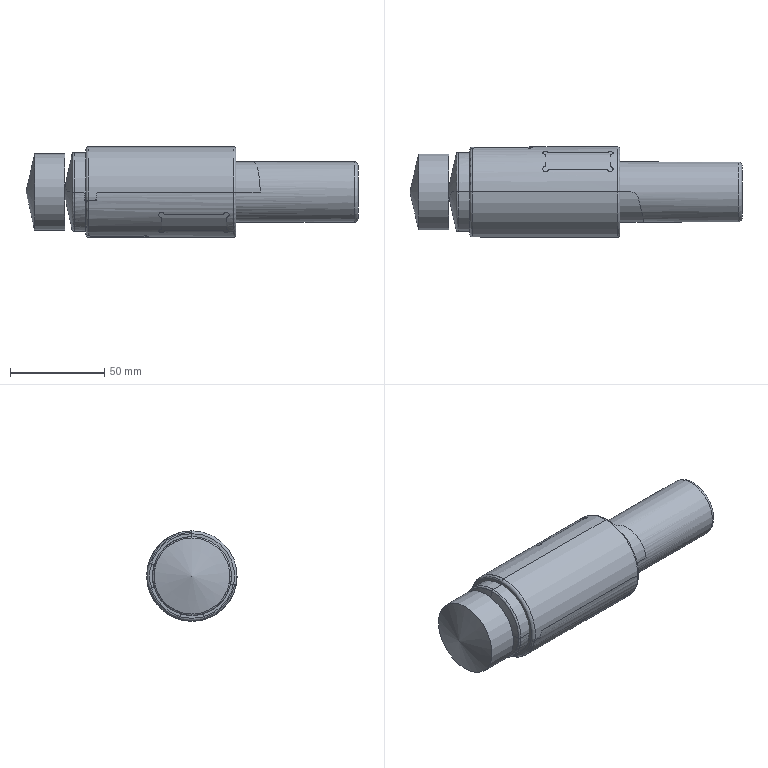NC program | NX | posted with a generic post | part box 176.413 x 48 x 48 mm
Lines 12628 to 12824 of 71815:
(FLOOR_WALL_1 , TOOL : D6JING)
N25182 T08 M6
N25184 G54
N25186 G17 G0 G90 X-61.329 Y-24.781 S6500 M3
N25188 G43 Z24.716 H8
N25190 Z3.
N25192 G94 G1 Z0. F500.
N25194 X-61.608 Y-24.298
N25196 G3 X-62.128 Y-23.998 R0.6
N25198 G1 X-150.97 F1000.
N25200 G2 X-154.682 Y-21.241 R3.999
N25202 G1 X-62.001
N25204 Y-18.999
N25206 X-54.673
N25208 X-54.797 Y-18.485
N25210 X-155.322
N25212 X-155.943 Y-15.728
N25214 X-55.46
N25216 X-55.563 Y-15.3
N25218 X-136.562
N25220 X-136.609 Y-15.306
N25222 X-136.652 Y-15.286
N25224 X-144.086 Y-12.971
N25226 G3 X-143.993 Y-13.564 R0.6
N25228 G1 Z3.
N25230 G0 Z32.265
N25232 X-126.191 Y-14.908 Z31.666
N25234 X-108.389 Y-16.227 Z31.011
N25236 X-90.587 Y-17.516 Z30.302
N25238 X-72.785 Y-18.775 Z29.538
N25240 X-54.982 Y-20. Z28.723
N25242 Z3.
N25244 G1 Z0. F500.
N25246 X-54.534 Y-19.574
N25248 G3 X-54.364 Y-18.999 R0.6
N25250 G1 X-55.326 Y-15. F1000.
N25252 X-136.562
N25254 X-144.182 Y-12.627
N25256 G3 X-144.485 Y-13.082 R1.266
N25258 G1 X-145.227 Y-15.
N25260 X-156.107
N25262 G3 X-156.626 Y-15.3 R0.6
N25264 G1 X-156.942 Y-15.847
N25266 Z3.
N25268 G0 Z31.207
(FLOOR_WALL_1_COPY , TOOL : D6JING)
N25270 X-100.58 Y26.407
N25272 Z22.972
N25274 Y16.85 Z13.415
N25276 G1 Y14.728 Z11.293 F500.
N25278 X-100.708 Y14.847 Z11.175
N25280 X-100.891 Y14.922 Z11.1
N25282 X-101.1 Y14.94 Z11.081
N25284 X-73.3 F1000.
N25286 Y13.01 Z13.011
N25288 X-101.1
N25290 Y11.08 Z14.941
N25292 X-73.3
N25294 X-73.327 Y11.228 Z14.794
N25296 X-73.433 Y11.358 Z14.664
N25298 X-73.6 Y11.448 Z14.574
N25300 X-73.15 Y10.897 Z15.125
N25302 X-73.063 Y10.939 Z15.082 F500.
N25304 X-73.009 Y11.005 Z15.016
N25306 X-73. Y11.08 Z14.941
N25308 Y15.153 Z10.868 F1000.
N25310 X-101.4
N25312 Y10.868 Z15.153
N25314 X-73.
N25316 Y11.08 Z14.941
N25318 X-73.027 Y11.228 Z14.794
N25320 X-73.133 Y11.358 Z14.664
N25322 X-73.3 Y11.448 Z14.574
N25324 X-74. Y11.734 Z14.288
N25326 Y13.855 Z16.409
N25328 G0 Y23.439 Z25.993
(FLOOR_WALL_1_COPY_COPY_1 , TOOL : D6JING)
N25330 X-100.58 Y-26.407
N25332 Z-22.972
N25334 Y-16.85 Z-13.415
N25336 G1 Y-14.728 Z-11.293 F500.
N25338 X-100.708 Y-14.847 Z-11.175
N25340 X-100.891 Y-14.922 Z-11.1
N25342 X-101.1 Y-14.94 Z-11.081
N25344 X-73.3 F1000.
N25346 Y-13.01 Z-13.011
N25348 X-101.1
N25350 Y-11.08 Z-14.941
N25352 X-73.3
N25354 X-73.327 Y-11.228 Z-14.794
N25356 X-73.433 Y-11.358 Z-14.664
N25358 X-73.6 Y-11.448 Z-14.574
N25360 X-73.15 Y-10.897 Z-15.125
N25362 X-73.063 Y-10.939 Z-15.082 F500.
N25364 X-73.009 Y-11.005 Z-15.016
N25366 X-73. Y-11.08 Z-14.941
N25368 Y-15.153 Z-10.868 F1000.
N25370 X-101.4
N25372 Y-10.868 Z-15.153
N25374 X-73.
N25376 Y-11.08 Z-14.941
N25378 X-73.027 Y-11.228 Z-14.794
N25380 X-73.133 Y-11.358 Z-14.664
N25382 X-73.3 Y-11.448 Z-14.574
N25384 X-74. Y-11.734 Z-14.288
N25386 Y-13.855 Z-16.409
N25388 G0 Y-23.439 Z-25.993
(FLOOR_WALL_1_COPY_COPY_2 , TOOL : D6JING)
N25390 X-100.58 Y22.972
N25392 Z-26.407
N25394 Y13.415 Z-16.85
N25396 G1 Y11.293 Z-14.728 F500.
N25398 X-100.708 Y11.175 Z-14.847
N25400 X-100.891 Y11.1 Z-14.922
N25402 X-101.1 Y11.081 Z-14.94
N25404 X-73.3 F1000.
N25406 Y13.011 Z-13.01
N25408 X-101.1
N25410 Y14.941 Z-11.08
N25412 X-73.3
N25414 X-73.327 Y14.794 Z-11.228
N25416 X-73.433 Y14.664 Z-11.358
N25418 X-73.6 Y14.574 Z-11.448
N25420 X-73.15 Y15.125 Z-10.897
N25422 X-73.063 Y15.082 Z-10.939 F500.
N25424 X-73.009 Y15.016 Z-11.005
N25426 X-73. Y14.941 Z-11.08
N25428 Y10.868 Z-15.153 F1000.
N25430 X-101.4
N25432 Y15.153 Z-10.868
N25434 X-73.
N25436 Y14.941 Z-11.08
N25438 X-73.027 Y14.794 Z-11.228
N25440 X-73.133 Y14.664 Z-11.358
N25442 X-73.3 Y14.574 Z-11.448
N25444 X-74. Y14.288 Z-11.734
N25446 Y16.409 Z-13.855
N25448 G0 Y25.993 Z-23.439
(FLOOR_WALL_1_COPY_COPY , TOOL : D6JING)
N25450 G18 Y34.971
N25452 X-116.569 Z1.424
N25454 Y23.4
N25456 G1 Y20.4 F500.
N25458 G3 X-116.05 Z1.724 R0.6
N25460 G1 X-140.05 F1000.
N25462 Z0.
N25464 X-116.05
N25466 Z-1.725
N25468 X-140.05
N25470 G3 X-139.75 Z-1.205 R0.6
N25472 G1 X-140.2 Z-1.985
N25474 G3 X-140.35 Z-1.725 R0.3 F500.
N25476 G1 Z2.025 F1000.
N25478 X-115.75
N25480 Z-2.025
N25482 X-140.35
N25484 Z-1.725
N25486 G3 X-140.05 Z-1.205 R0.6
N25488 G1 X-139.35 Z-0.801
N25490 Y23.4
N25492 G0 Y34.991
(FLOOR_WALL_1_COPY_COPY_COPY , TOOL : D6JING)
N25494 G17 X-116.569 Y1.424
N25496 Z-34.971
N25498 Z-23.4
N25500 G1 Z-20.4 F500.
N25502 G2 X-116.05 Y1.724 R0.6
N25504 G1 X-140.05 F1000.
N25506 Y0.
N25508 X-116.05
N25510 Y-1.725
N25512 X-140.05
N25514 G2 X-139.75 Y-1.205 R0.6
N25516 G1 X-140.2 Y-1.985
N25518 G2 X-140.35 Y-1.725 R0.3 F500.
N25520 G1 Y2.025 F1000.
N25522 X-115.75
N25524 Y-2.025
N25526 X-140.35
N25528 Y-1.725
N25530 G2 X-140.05 Y-1.205 R0.6
N25532 G1 X-139.35 Y-0.801
N25534 Z-23.4
N25536 G0 Z-34.991
N25538 M5